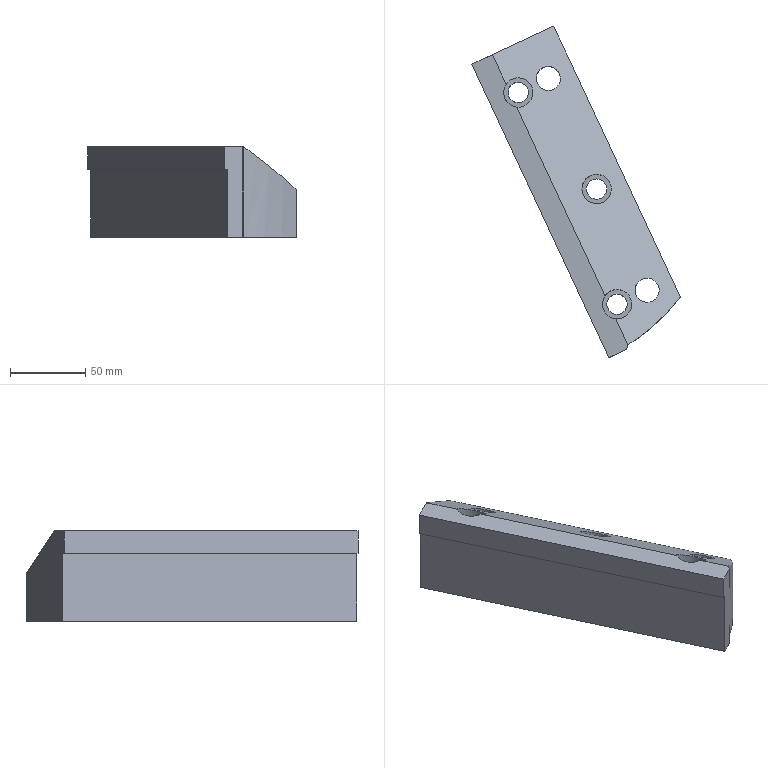Part | NX | features solid 2 | 1 solid | 23 faces | box 138.174 x 220.213 x 60 mm | volume 552475 mm3 | plane 13 | cylinder 8 | spline 2 | commonest cylinder face diameters 13.5 x3 19.5 x3 16 x2